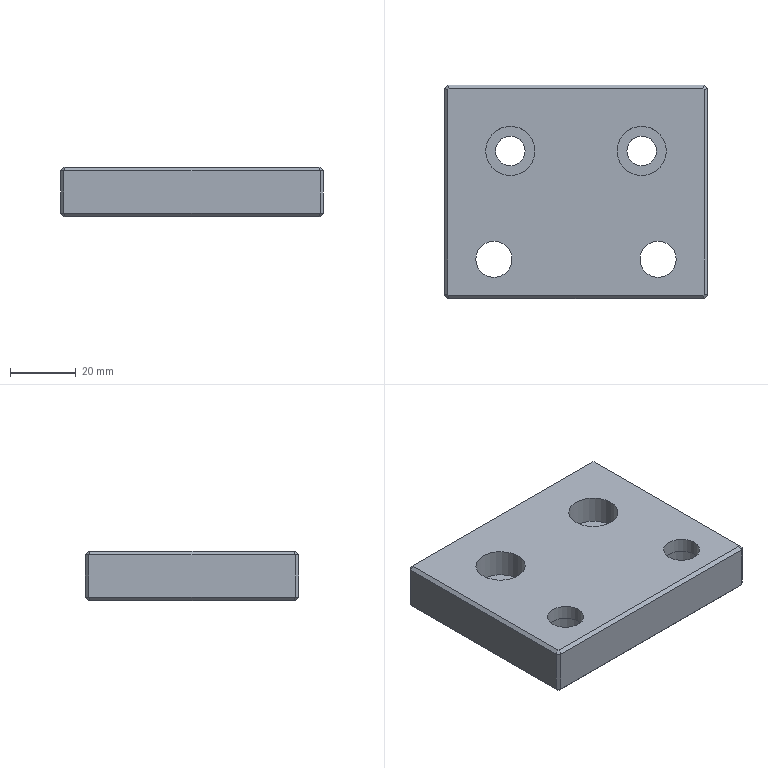Part | NX | 1 solid | 38 faces | box 80 x 65 x 15 mm | volume 67600 mm3 | plane 30 | cylinder 8 | commonest cylinder face diameters 9 x2 11 x2 15 x2 18 x2
STEP:
#1=CARTESIAN_POINT('',(40.,19.,1.));
#2=VERTEX_POINT('',#1);
#3=CARTESIAN_POINT('',(40.,19.,14.));
#4=VERTEX_POINT('',#3);
#5=CARTESIAN_POINT('',(40.,19.,15.));
#6=DIRECTION('',(0.,0.,1.));
#7=VECTOR('',#6,1000.);
#8=LINE('',#5,#7);
#9=EDGE_CURVE('',#2,#4,#8,.T.);
#10=ORIENTED_EDGE('',*,*,#9,.T.);
#11=CARTESIAN_POINT('',(40.,-44.,14.));
#12=VERTEX_POINT('',#11);
#13=CARTESIAN_POINT('',(40.,20.,14.));
#14=DIRECTION('',(0.,-1.,0.));
#15=VECTOR('',#14,1000.);
#16=LINE('',#13,#15);
#17=EDGE_CURVE('',#4,#12,#16,.T.);
#18=ORIENTED_EDGE('',*,*,#17,.T.);
#19=CARTESIAN_POINT('',(40.,-44.,1.));
#20=VERTEX_POINT('',#19);
#21=CARTESIAN_POINT('',(40.,-44.,15.));
#22=DIRECTION('',(0.,0.,-1.));
#23=VECTOR('',#22,1000.);
#24=LINE('',#21,#23);
#25=EDGE_CURVE('',#12,#20,#24,.T.);
#26=ORIENTED_EDGE('',*,*,#25,.T.);
#27=CARTESIAN_POINT('',(40.,19.,1.));
#28=DIRECTION('',(0.,1.,0.));
#29=VECTOR('',#28,1000.);
#30=LINE('',#27,#29);
#31=EDGE_CURVE('',#20,#2,#30,.T.);
#32=ORIENTED_EDGE('',*,*,#31,.T.);
#33=EDGE_LOOP('',(#10,#18,#26,#32));
#34=FACE_BOUND('',#33,.T.);
#35=CARTESIAN_POINT('',(40.,20.,15.));
#36=DIRECTION('',(-1.,0.,0.));
#37=DIRECTION('',(0.,-1.,0.));
#38=AXIS2_PLACEMENT_3D('',#35,#36,#37);
#39=PLANE('',#38);
#40=ADVANCED_FACE('',(#34),#39,.F.);
#41=CARTESIAN_POINT('',(-39.,20.,1.));
#42=VERTEX_POINT('',#41);
#43=CARTESIAN_POINT('',(-39.,20.,14.));
#44=VERTEX_POINT('',#43);
#45=CARTESIAN_POINT('',(-39.,20.,15.));
#46=DIRECTION('',(0.,0.,1.));
#47=VECTOR('',#46,1000.);
#48=LINE('',#45,#47);
#49=EDGE_CURVE('',#42,#44,#48,.T.);
#50=ORIENTED_EDGE('',*,*,#49,.T.);
#51=CARTESIAN_POINT('',(39.,20.,14.));
#52=VERTEX_POINT('',#51);
#53=CARTESIAN_POINT('',(40.,20.,14.));
#54=DIRECTION('',(1.,0.,0.));
#55=VECTOR('',#54,1000.);
#56=LINE('',#53,#55);
#57=EDGE_CURVE('',#44,#52,#56,.T.);
#58=ORIENTED_EDGE('',*,*,#57,.T.);
#59=CARTESIAN_POINT('',(39.,20.,1.));
#60=VERTEX_POINT('',#59);
#61=CARTESIAN_POINT('',(39.,20.,15.));
#62=DIRECTION('',(0.,0.,-1.));
#63=VECTOR('',#62,1000.);
#64=LINE('',#61,#63);
#65=EDGE_CURVE('',#52,#60,#64,.T.);
#66=ORIENTED_EDGE('',*,*,#65,.T.);
#67=CARTESIAN_POINT('',(-39.,20.,1.));
#68=DIRECTION('',(-1.,0.,0.));
#69=VECTOR('',#68,1000.);
#70=LINE('',#67,#69);
#71=EDGE_CURVE('',#60,#42,#70,.T.);
#72=ORIENTED_EDGE('',*,*,#71,.T.);
#73=EDGE_LOOP('',(#50,#58,#66,#72));
#74=FACE_BOUND('',#73,.T.);
#75=CARTESIAN_POINT('',(40.,20.,15.));
#76=DIRECTION('',(0.,-1.,0.));
#77=DIRECTION('',(0.,0.,-1.));
#78=AXIS2_PLACEMENT_3D('',#75,#76,#77);
#79=PLANE('',#78);
#80=ADVANCED_FACE('',(#74),#79,.F.);
#81=CARTESIAN_POINT('',(-40.,-44.,1.));
#82=VERTEX_POINT('',#81);
#83=CARTESIAN_POINT('',(-40.,-44.,14.));
#84=VERTEX_POINT('',#83);
#85=CARTESIAN_POINT('',(-40.,-44.,15.));
#86=DIRECTION('',(0.,0.,1.));
#87=VECTOR('',#86,1000.);
#88=LINE('',#85,#87);
#89=EDGE_CURVE('',#82,#84,#88,.T.);
#90=ORIENTED_EDGE('',*,*,#89,.T.);
#91=CARTESIAN_POINT('',(-40.,19.,14.));
#92=VERTEX_POINT('',#91);
#93=CARTESIAN_POINT('',(-40.,20.,14.));
#94=DIRECTION('',(0.,1.,0.));
#95=VECTOR('',#94,1000.);
#96=LINE('',#93,#95);
#97=EDGE_CURVE('',#84,#92,#96,.T.);
#98=ORIENTED_EDGE('',*,*,#97,.T.);
#99=CARTESIAN_POINT('',(-40.,19.,1.));
#100=VERTEX_POINT('',#99);
#101=CARTESIAN_POINT('',(-40.,19.,15.));
#102=DIRECTION('',(0.,0.,-1.));
#103=VECTOR('',#102,1000.);
#104=LINE('',#101,#103);
#105=EDGE_CURVE('',#92,#100,#104,.T.);
#106=ORIENTED_EDGE('',*,*,#105,.T.);
#107=CARTESIAN_POINT('',(-40.,-44.,1.));
#108=DIRECTION('',(0.,-1.,0.));
#109=VECTOR('',#108,1000.);
#110=LINE('',#107,#109);
#111=EDGE_CURVE('',#100,#82,#110,.T.);
#112=ORIENTED_EDGE('',*,*,#111,.T.);
#113=EDGE_LOOP('',(#90,#98,#106,#112));
#114=FACE_BOUND('',#113,.T.);
#115=CARTESIAN_POINT('',(-40.,20.,15.));
#116=DIRECTION('',(1.,0.,0.));
#117=DIRECTION('',(0.,1.,0.));
#118=AXIS2_PLACEMENT_3D('',#115,#116,#117);
#119=PLANE('',#118);
#120=ADVANCED_FACE('',(#114),#119,.F.);
#121=CARTESIAN_POINT('',(39.,-45.,1.));
#122=VERTEX_POINT('',#121);
#123=CARTESIAN_POINT('',(39.,-45.,14.));
#124=VERTEX_POINT('',#123);
#125=CARTESIAN_POINT('',(39.,-45.,15.));
#126=DIRECTION('',(0.,0.,1.));
#127=VECTOR('',#126,1000.);
#128=LINE('',#125,#127);
#129=EDGE_CURVE('',#122,#124,#128,.T.);
#130=ORIENTED_EDGE('',*,*,#129,.T.);
#131=CARTESIAN_POINT('',(-39.,-45.,14.));
#132=VERTEX_POINT('',#131);
#133=CARTESIAN_POINT('',(40.,-45.,14.));
#134=DIRECTION('',(-1.,0.,0.));
#135=VECTOR('',#134,1000.);
#136=LINE('',#133,#135);
#137=EDGE_CURVE('',#124,#132,#136,.T.);
#138=ORIENTED_EDGE('',*,*,#137,.T.);
#139=CARTESIAN_POINT('',(-39.,-45.,1.));
#140=VERTEX_POINT('',#139);
#141=CARTESIAN_POINT('',(-39.,-45.,15.));
#142=DIRECTION('',(0.,0.,-1.));
#143=VECTOR('',#142,1000.);
#144=LINE('',#141,#143);
#145=EDGE_CURVE('',#132,#140,#144,.T.);
#146=ORIENTED_EDGE('',*,*,#145,.T.);
#147=CARTESIAN_POINT('',(39.,-45.,1.));
#148=DIRECTION('',(1.,0.,0.));
#149=VECTOR('',#148,1000.);
#150=LINE('',#147,#149);
#151=EDGE_CURVE('',#140,#122,#150,.T.);
#152=ORIENTED_EDGE('',*,*,#151,.T.);
#153=EDGE_LOOP('',(#130,#138,#146,#152));
#154=FACE_BOUND('',#153,.T.);
#155=CARTESIAN_POINT('',(40.,-45.,15.));
#156=DIRECTION('',(0.,1.,0.));
#157=DIRECTION('',(0.,0.,1.));
#158=AXIS2_PLACEMENT_3D('',#155,#156,#157);
#159=PLANE('',#158);
#160=ADVANCED_FACE('',(#154),#159,.F.);
#161=CARTESIAN_POINT('',(-38.586,-44.,15.));
#162=VERTEX_POINT('',#161);
#163=CARTESIAN_POINT('',(38.586,-44.,15.));
#164=VERTEX_POINT('',#163);
#165=CARTESIAN_POINT('',(0.,-44.,15.));
#166=DIRECTION('',(1.,0.,0.));
#167=VECTOR('',#166,1000.);
#168=LINE('',#165,#167);
#169=EDGE_CURVE('',#162,#164,#168,.T.);
#170=ORIENTED_EDGE('',*,*,#169,.T.);
#171=CARTESIAN_POINT('',(39.,-43.586,15.));
#172=VERTEX_POINT('',#171);
#173=CARTESIAN_POINT('',(39.293,-43.293,15.));
#174=DIRECTION('',(0.7071,0.7071,0.));
#175=VECTOR('',#174,1000.);
#176=LINE('',#173,#175);
#177=EDGE_CURVE('',#164,#172,#176,.T.);
#178=ORIENTED_EDGE('',*,*,#177,.T.);
#179=CARTESIAN_POINT('',(39.,18.586,15.));
#180=VERTEX_POINT('',#179);
#181=CARTESIAN_POINT('',(39.,0.,15.));
#182=DIRECTION('',(0.,1.,0.));
#183=VECTOR('',#182,1000.);
#184=LINE('',#181,#183);
#185=EDGE_CURVE('',#172,#180,#184,.T.);
#186=ORIENTED_EDGE('',*,*,#185,.T.);
#187=CARTESIAN_POINT('',(38.586,19.,15.));
#188=VERTEX_POINT('',#187);
#189=CARTESIAN_POINT('',(38.293,19.293,15.));
#190=DIRECTION('',(-0.7071,0.7071,0.));
#191=VECTOR('',#190,1000.);
#192=LINE('',#189,#191);
#193=EDGE_CURVE('',#180,#188,#192,.T.);
#194=ORIENTED_EDGE('',*,*,#193,.T.);
#195=CARTESIAN_POINT('',(-38.586,19.,15.));
#196=VERTEX_POINT('',#195);
#197=CARTESIAN_POINT('',(0.,19.,15.));
#198=DIRECTION('',(-1.,0.,0.));
#199=VECTOR('',#198,1000.);
#200=LINE('',#197,#199);
#201=EDGE_CURVE('',#188,#196,#200,.T.);
#202=ORIENTED_EDGE('',*,*,#201,.T.);
#203=CARTESIAN_POINT('',(-39.,18.586,15.));
#204=VERTEX_POINT('',#203);
#205=CARTESIAN_POINT('',(-39.293,18.293,15.));
#206=DIRECTION('',(-0.7071,-0.7071,0.));
#207=VECTOR('',#206,1000.);
#208=LINE('',#205,#207);
#209=EDGE_CURVE('',#196,#204,#208,.T.);
#210=ORIENTED_EDGE('',*,*,#209,.T.);
#211=CARTESIAN_POINT('',(-39.,-43.586,15.));
#212=VERTEX_POINT('',#211);
#213=CARTESIAN_POINT('',(-39.,0.,15.));
#214=DIRECTION('',(0.,-1.,0.));
#215=VECTOR('',#214,1000.);
#216=LINE('',#213,#215);
#217=EDGE_CURVE('',#204,#212,#216,.T.);
#218=ORIENTED_EDGE('',*,*,#217,.T.);
#219=CARTESIAN_POINT('',(-38.293,-44.293,15.));
#220=DIRECTION('',(0.7071,-0.7071,0.));
#221=VECTOR('',#220,1000.);
#222=LINE('',#219,#221);
#223=EDGE_CURVE('',#212,#162,#222,.T.);
#224=ORIENTED_EDGE('',*,*,#223,.T.);
#225=EDGE_LOOP('',(#170,#178,#186,#194,#202,#210,#218,#224));
#226=FACE_BOUND('',#225,.T.);
#227=CARTESIAN_POINT('',(19.5,-33.,15.));
#228=VERTEX_POINT('',#227);
#229=CARTESIAN_POINT('',(25.,-33.,15.));
#230=DIRECTION('',(0.,0.,-1.));
#231=DIRECTION('',(-1.,0.,0.));
#232=AXIS2_PLACEMENT_3D('',#229,#230,#231);
#233=CIRCLE('',#232,5.5);
#234=EDGE_CURVE('',#228,#228,#233,.T.);
#235=ORIENTED_EDGE('',*,*,#234,.T.);
#236=EDGE_LOOP('',(#235));
#237=FACE_BOUND('',#236,.T.);
#238=CARTESIAN_POINT('',(-30.5,-33.,15.));
#239=VERTEX_POINT('',#238);
#240=CARTESIAN_POINT('',(-25.,-33.,15.));
#241=DIRECTION('',(0.,0.,-1.));
#242=DIRECTION('',(-1.,0.,0.));
#243=AXIS2_PLACEMENT_3D('',#240,#241,#242);
#244=CIRCLE('',#243,5.5);
#245=EDGE_CURVE('',#239,#239,#244,.T.);
#246=ORIENTED_EDGE('',*,*,#245,.T.);
#247=EDGE_LOOP('',(#246));
#248=FACE_BOUND('',#247,.T.);
#249=CARTESIAN_POINT('',(-12.5,0.,15.));
#250=VERTEX_POINT('',#249);
#251=CARTESIAN_POINT('',(-20.,0.,15.));
#252=DIRECTION('',(0.,0.,1.));
#253=DIRECTION('',(1.,0.,0.));
#254=AXIS2_PLACEMENT_3D('',#251,#252,#253);
#255=CIRCLE('',#254,7.5);
#256=EDGE_CURVE('',#250,#250,#255,.T.);
#257=ORIENTED_EDGE('',*,*,#256,.F.);
#258=EDGE_LOOP('',(#257));
#259=FACE_BOUND('',#258,.T.);
#260=CARTESIAN_POINT('',(27.5,0.,15.));
#261=VERTEX_POINT('',#260);
#262=CARTESIAN_POINT('',(20.,0.,15.));
#263=DIRECTION('',(0.,0.,1.));
#264=DIRECTION('',(1.,0.,0.));
#265=AXIS2_PLACEMENT_3D('',#262,#263,#264);
#266=CIRCLE('',#265,7.5);
#267=EDGE_CURVE('',#261,#261,#266,.T.);
#268=ORIENTED_EDGE('',*,*,#267,.F.);
#269=EDGE_LOOP('',(#268));
#270=FACE_BOUND('',#269,.T.);
#271=CARTESIAN_POINT('',(0.,0.,15.));
#272=DIRECTION('',(0.,0.,-1.));
#273=DIRECTION('',(-1.,0.,0.));
#274=AXIS2_PLACEMENT_3D('',#271,#272,#273);
#275=PLANE('',#274);
#276=ADVANCED_FACE('',(#226,#237,#248,#259,#270),#275,.F.);
#277=CARTESIAN_POINT('',(-38.586,19.,0.));
#278=VERTEX_POINT('',#277);
#279=CARTESIAN_POINT('',(38.586,19.,0.));
#280=VERTEX_POINT('',#279);
#281=CARTESIAN_POINT('',(39.,19.,0.));
#282=DIRECTION('',(1.,0.,0.));
#283=VECTOR('',#282,1000.);
#284=LINE('',#281,#283);
#285=EDGE_CURVE('',#278,#280,#284,.T.);
#286=ORIENTED_EDGE('',*,*,#285,.T.);
#287=CARTESIAN_POINT('',(39.,18.586,0.));
#288=VERTEX_POINT('',#287);
#289=CARTESIAN_POINT('',(28.793,28.793,0.));
#290=DIRECTION('',(0.7071,-0.7071,0.));
#291=VECTOR('',#290,1000.);
#292=LINE('',#289,#291);
#293=EDGE_CURVE('',#280,#288,#292,.T.);
#294=ORIENTED_EDGE('',*,*,#293,.T.);
#295=CARTESIAN_POINT('',(39.,-43.586,0.));
#296=VERTEX_POINT('',#295);
#297=CARTESIAN_POINT('',(39.,-44.,0.));
#298=DIRECTION('',(0.,-1.,0.));
#299=VECTOR('',#298,1000.);
#300=LINE('',#297,#299);
#301=EDGE_CURVE('',#288,#296,#300,.T.);
#302=ORIENTED_EDGE('',*,*,#301,.T.);
#303=CARTESIAN_POINT('',(38.586,-44.,0.));
#304=VERTEX_POINT('',#303);
#305=CARTESIAN_POINT('',(41.293,-41.293,0.));
#306=DIRECTION('',(-0.7071,-0.7071,0.));
#307=VECTOR('',#306,1000.);
#308=LINE('',#305,#307);
#309=EDGE_CURVE('',#296,#304,#308,.T.);
#310=ORIENTED_EDGE('',*,*,#309,.T.);
#311=CARTESIAN_POINT('',(-38.586,-44.,0.));
#312=VERTEX_POINT('',#311);
#313=CARTESIAN_POINT('',(-39.,-44.,0.));
#314=DIRECTION('',(-1.,0.,0.));
#315=VECTOR('',#314,1000.);
#316=LINE('',#313,#315);
#317=EDGE_CURVE('',#304,#312,#316,.T.);
#318=ORIENTED_EDGE('',*,*,#317,.T.);
#319=CARTESIAN_POINT('',(-39.,-43.586,0.));
#320=VERTEX_POINT('',#319);
#321=CARTESIAN_POINT('',(-41.293,-41.293,0.));
#322=DIRECTION('',(-0.7071,0.7071,0.));
#323=VECTOR('',#322,1000.);
#324=LINE('',#321,#323);
#325=EDGE_CURVE('',#312,#320,#324,.T.);
#326=ORIENTED_EDGE('',*,*,#325,.T.);
#327=CARTESIAN_POINT('',(-39.,18.586,0.));
#328=VERTEX_POINT('',#327);
#329=CARTESIAN_POINT('',(-39.,19.,0.));
#330=DIRECTION('',(0.,1.,0.));
#331=VECTOR('',#330,1000.);
#332=LINE('',#329,#331);
#333=EDGE_CURVE('',#320,#328,#332,.T.);
#334=ORIENTED_EDGE('',*,*,#333,.T.);
#335=CARTESIAN_POINT('',(-28.793,28.793,0.));
#336=DIRECTION('',(0.7071,0.7071,0.));
#337=VECTOR('',#336,1000.);
#338=LINE('',#335,#337);
#339=EDGE_CURVE('',#328,#278,#338,.T.);
#340=ORIENTED_EDGE('',*,*,#339,.T.);
#341=EDGE_LOOP('',(#286,#294,#302,#310,#318,#326,#334,#340));
#342=FACE_BOUND('',#341,.T.);
#343=CARTESIAN_POINT('',(16.,-33.,0.));
#344=VERTEX_POINT('',#343);
#345=CARTESIAN_POINT('',(25.,-33.,0.));
#346=DIRECTION('',(0.,0.,-1.));
#347=DIRECTION('',(-1.,0.,0.));
#348=AXIS2_PLACEMENT_3D('',#345,#346,#347);
#349=CIRCLE('',#348,9.);
#350=EDGE_CURVE('',#344,#344,#349,.T.);
#351=ORIENTED_EDGE('',*,*,#350,.F.);
#352=EDGE_LOOP('',(#351));
#353=FACE_BOUND('',#352,.T.);
#354=CARTESIAN_POINT('',(-34.,-33.,0.));
#355=VERTEX_POINT('',#354);
#356=CARTESIAN_POINT('',(-25.,-33.,0.));
#357=DIRECTION('',(0.,0.,-1.));
#358=DIRECTION('',(-1.,0.,0.));
#359=AXIS2_PLACEMENT_3D('',#356,#357,#358);
#360=CIRCLE('',#359,9.);
#361=EDGE_CURVE('',#355,#355,#360,.T.);
#362=ORIENTED_EDGE('',*,*,#361,.F.);
#363=EDGE_LOOP('',(#362));
#364=FACE_BOUND('',#363,.T.);
#365=CARTESIAN_POINT('',(-15.5,0.,0.));
#366=VERTEX_POINT('',#365);
#367=CARTESIAN_POINT('',(-20.,0.,0.));
#368=DIRECTION('',(0.,0.,1.));
#369=DIRECTION('',(1.,0.,0.));
#370=AXIS2_PLACEMENT_3D('',#367,#368,#369);
#371=CIRCLE('',#370,4.5);
#372=EDGE_CURVE('',#366,#366,#371,.T.);
#373=ORIENTED_EDGE('',*,*,#372,.T.);
#374=EDGE_LOOP('',(#373));
#375=FACE_BOUND('',#374,.T.);
#376=CARTESIAN_POINT('',(24.5,0.,0.));
#377=VERTEX_POINT('',#376);
#378=CARTESIAN_POINT('',(20.,0.,0.));
#379=DIRECTION('',(0.,0.,1.));
#380=DIRECTION('',(1.,0.,0.));
#381=AXIS2_PLACEMENT_3D('',#378,#379,#380);
#382=CIRCLE('',#381,4.5);
#383=EDGE_CURVE('',#377,#377,#382,.T.);
#384=ORIENTED_EDGE('',*,*,#383,.T.);
#385=EDGE_LOOP('',(#384));
#386=FACE_BOUND('',#385,.T.);
#387=CARTESIAN_POINT('',(0.,0.,0.));
#388=DIRECTION('',(0.,0.,-1.));
#389=DIRECTION('',(-1.,0.,0.));
#390=AXIS2_PLACEMENT_3D('',#387,#388,#389);
#391=PLANE('',#390);
#392=ADVANCED_FACE('',(#342,#353,#364,#375,#386),#391,.T.);
#393=ORIENTED_EDGE('',*,*,#383,.F.);
#394=EDGE_LOOP('',(#393));
#395=FACE_BOUND('',#394,.T.);
#396=CARTESIAN_POINT('',(24.5,0.,6.4));
#397=VERTEX_POINT('',#396);
#398=CARTESIAN_POINT('',(20.,0.,6.4));
#399=DIRECTION('',(0.,0.,1.));
#400=DIRECTION('',(1.,0.,0.));
#401=AXIS2_PLACEMENT_3D('',#398,#399,#400);
#402=CIRCLE('',#401,4.5);
#403=EDGE_CURVE('',#397,#397,#402,.T.);
#404=ORIENTED_EDGE('',*,*,#403,.T.);
#405=EDGE_LOOP('',(#404));
#406=FACE_BOUND('',#405,.T.);
#407=CARTESIAN_POINT('',(20.,0.,15.));
#408=DIRECTION('',(0.,0.,1.));
#409=DIRECTION('',(1.,0.,0.));
#410=AXIS2_PLACEMENT_3D('',#407,#408,#409);
#411=CYLINDRICAL_SURFACE('',#410,4.5);
#412=ADVANCED_FACE('',(#395,#406),#411,.F.);
#413=ORIENTED_EDGE('',*,*,#403,.F.);
#414=EDGE_LOOP('',(#413));
#415=FACE_BOUND('',#414,.T.);
#416=CARTESIAN_POINT('',(27.5,0.,6.4));
#417=VERTEX_POINT('',#416);
#418=CARTESIAN_POINT('',(20.,0.,6.4));
#419=DIRECTION('',(0.,0.,1.));
#420=DIRECTION('',(1.,0.,0.));
#421=AXIS2_PLACEMENT_3D('',#418,#419,#420);
#422=CIRCLE('',#421,7.5);
#423=EDGE_CURVE('',#417,#417,#422,.T.);
#424=ORIENTED_EDGE('',*,*,#423,.T.);
#425=EDGE_LOOP('',(#424));
#426=FACE_BOUND('',#425,.T.);
#427=CARTESIAN_POINT('',(24.5,0.,6.4));
#428=DIRECTION('',(0.,0.,-1.));
#429=DIRECTION('',(-1.,0.,0.));
#430=AXIS2_PLACEMENT_3D('',#427,#428,#429);
#431=PLANE('',#430);
#432=ADVANCED_FACE('',(#415,#426),#431,.F.);
#433=ORIENTED_EDGE('',*,*,#423,.F.);
#434=EDGE_LOOP('',(#433));
#435=FACE_BOUND('',#434,.T.);
#436=ORIENTED_EDGE('',*,*,#267,.T.);
#437=EDGE_LOOP('',(#436));
#438=FACE_BOUND('',#437,.T.);
#439=CARTESIAN_POINT('',(20.,0.,15.));
#440=DIRECTION('',(0.,0.,1.));
#441=DIRECTION('',(1.,0.,0.));
#442=AXIS2_PLACEMENT_3D('',#439,#440,#441);
#443=CYLINDRICAL_SURFACE('',#442,7.5);
#444=ADVANCED_FACE('',(#435,#438),#443,.F.);
#445=ORIENTED_EDGE('',*,*,#372,.F.);
#446=EDGE_LOOP('',(#445));
#447=FACE_BOUND('',#446,.T.);
#448=CARTESIAN_POINT('',(-15.5,0.,6.4));
#449=VERTEX_POINT('',#448);
#450=CARTESIAN_POINT('',(-20.,0.,6.4));
#451=DIRECTION('',(0.,0.,1.));
#452=DIRECTION('',(1.,0.,0.));
#453=AXIS2_PLACEMENT_3D('',#450,#451,#452);
#454=CIRCLE('',#453,4.5);
#455=EDGE_CURVE('',#449,#449,#454,.T.);
#456=ORIENTED_EDGE('',*,*,#455,.T.);
#457=EDGE_LOOP('',(#456));
#458=FACE_BOUND('',#457,.T.);
#459=CARTESIAN_POINT('',(-20.,0.,15.));
#460=DIRECTION('',(0.,0.,1.));
#461=DIRECTION('',(1.,0.,0.));
#462=AXIS2_PLACEMENT_3D('',#459,#460,#461);
#463=CYLINDRICAL_SURFACE('',#462,4.5);
#464=ADVANCED_FACE('',(#447,#458),#463,.F.);
#465=ORIENTED_EDGE('',*,*,#455,.F.);
#466=EDGE_LOOP('',(#465));
#467=FACE_BOUND('',#466,.T.);
#468=CARTESIAN_POINT('',(-12.5,0.,6.4));
#469=VERTEX_POINT('',#468);
#470=CARTESIAN_POINT('',(-20.,0.,6.4));
#471=DIRECTION('',(0.,0.,1.));
#472=DIRECTION('',(1.,0.,0.));
#473=AXIS2_PLACEMENT_3D('',#470,#471,#472);
#474=CIRCLE('',#473,7.5);
#475=EDGE_CURVE('',#469,#469,#474,.T.);
#476=ORIENTED_EDGE('',*,*,#475,.T.);
#477=EDGE_LOOP('',(#476));
#478=FACE_BOUND('',#477,.T.);
#479=CARTESIAN_POINT('',(-15.5,0.,6.4));
#480=DIRECTION('',(0.,0.,-1.));
#481=DIRECTION('',(-1.,0.,0.));
#482=AXIS2_PLACEMENT_3D('',#479,#480,#481);
#483=PLANE('',#482);
#484=ADVANCED_FACE('',(#467,#478),#483,.F.);
#485=ORIENTED_EDGE('',*,*,#475,.F.);
#486=EDGE_LOOP('',(#485));
#487=FACE_BOUND('',#486,.T.);
#488=ORIENTED_EDGE('',*,*,#256,.T.);
#489=EDGE_LOOP('',(#488));
#490=FACE_BOUND('',#489,.T.);
#491=CARTESIAN_POINT('',(-20.,0.,15.));
#492=DIRECTION('',(0.,0.,1.));
#493=DIRECTION('',(1.,0.,0.));
#494=AXIS2_PLACEMENT_3D('',#491,#492,#493);
#495=CYLINDRICAL_SURFACE('',#494,7.5);
#496=ADVANCED_FACE('',(#487,#490),#495,.F.);
#497=ORIENTED_EDGE('',*,*,#245,.F.);
#498=EDGE_LOOP('',(#497));
#499=FACE_BOUND('',#498,.T.);
#500=CARTESIAN_POINT('',(-30.5,-33.,10.6));
#501=VERTEX_POINT('',#500);
#502=CARTESIAN_POINT('',(-25.,-33.,10.6));
#503=DIRECTION('',(0.,0.,-1.));
#504=DIRECTION('',(-1.,0.,0.));
#505=AXIS2_PLACEMENT_3D('',#502,#503,#504);
#506=CIRCLE('',#505,5.5);
#507=EDGE_CURVE('',#501,#501,#506,.T.);
#508=ORIENTED_EDGE('',*,*,#507,.T.);
#509=EDGE_LOOP('',(#508));
#510=FACE_BOUND('',#509,.T.);
#511=CARTESIAN_POINT('',(-25.,-33.,0.));
#512=DIRECTION('',(0.,0.,-1.));
#513=DIRECTION('',(-1.,0.,0.));
#514=AXIS2_PLACEMENT_3D('',#511,#512,#513);
#515=CYLINDRICAL_SURFACE('',#514,5.5);
#516=ADVANCED_FACE('',(#499,#510),#515,.F.);
#517=ORIENTED_EDGE('',*,*,#507,.F.);
#518=EDGE_LOOP('',(#517));
#519=FACE_BOUND('',#518,.T.);
#520=CARTESIAN_POINT('',(-34.,-33.,10.6));
#521=VERTEX_POINT('',#520);
#522=CARTESIAN_POINT('',(-25.,-33.,10.6));
#523=DIRECTION('',(0.,0.,-1.));
#524=DIRECTION('',(-1.,0.,0.));
#525=AXIS2_PLACEMENT_3D('',#522,#523,#524);
#526=CIRCLE('',#525,9.);
#527=EDGE_CURVE('',#521,#521,#526,.T.);
#528=ORIENTED_EDGE('',*,*,#527,.T.);
#529=EDGE_LOOP('',(#528));
#530=FACE_BOUND('',#529,.T.);
#531=CARTESIAN_POINT('',(-19.5,-33.,10.6));
#532=DIRECTION('',(0.,0.,1.));
#533=DIRECTION('',(1.,0.,0.));
#534=AXIS2_PLACEMENT_3D('',#531,#532,#533);
#535=PLANE('',#534);
#536=ADVANCED_FACE('',(#519,#530),#535,.F.);
#537=ORIENTED_EDGE('',*,*,#527,.F.);
#538=EDGE_LOOP('',(#537));
#539=FACE_BOUND('',#538,.T.);
#540=ORIENTED_EDGE('',*,*,#361,.T.);
#541=EDGE_LOOP('',(#540));
#542=FACE_BOUND('',#541,.T.);
#543=CARTESIAN_POINT('',(-25.,-33.,0.));
#544=DIRECTION('',(0.,0.,-1.));
#545=DIRECTION('',(-1.,0.,0.));
#546=AXIS2_PLACEMENT_3D('',#543,#544,#545);
#547=CYLINDRICAL_SURFACE('',#546,9.);
#548=ADVANCED_FACE('',(#539,#542),#547,.F.);
#549=ORIENTED_EDGE('',*,*,#234,.F.);
#550=EDGE_LOOP('',(#549));
#551=FACE_BOUND('',#550,.T.);
#552=CARTESIAN_POINT('',(19.5,-33.,10.6));
#553=VERTEX_POINT('',#552);
#554=CARTESIAN_POINT('',(25.,-33.,10.6));
#555=DIRECTION('',(0.,0.,-1.));
#556=DIRECTION('',(-1.,0.,0.));
#557=AXIS2_PLACEMENT_3D('',#554,#555,#556);
#558=CIRCLE('',#557,5.5);
#559=EDGE_CURVE('',#553,#553,#558,.T.);
#560=ORIENTED_EDGE('',*,*,#559,.T.);
#561=EDGE_LOOP('',(#560));
#562=FACE_BOUND('',#561,.T.);
#563=CARTESIAN_POINT('',(25.,-33.,0.));
#564=DIRECTION('',(0.,0.,-1.));
#565=DIRECTION('',(-1.,0.,0.));
#566=AXIS2_PLACEMENT_3D('',#563,#564,#565);
#567=CYLINDRICAL_SURFACE('',#566,5.5);
#568=ADVANCED_FACE('',(#551,#562),#567,.F.);
#569=ORIENTED_EDGE('',*,*,#559,.F.);
#570=EDGE_LOOP('',(#569));
#571=FACE_BOUND('',#570,.T.);
#572=CARTESIAN_POINT('',(16.,-33.,10.6));
#573=VERTEX_POINT('',#572);
#574=CARTESIAN_POINT('',(25.,-33.,10.6));
#575=DIRECTION('',(0.,0.,-1.));
#576=DIRECTION('',(-1.,0.,0.));
#577=AXIS2_PLACEMENT_3D('',#574,#575,#576);
#578=CIRCLE('',#577,9.);
#579=EDGE_CURVE('',#573,#573,#578,.T.);
#580=ORIENTED_EDGE('',*,*,#579,.T.);
#581=EDGE_LOOP('',(#580));
#582=FACE_BOUND('',#581,.T.);
#583=CARTESIAN_POINT('',(30.5,-33.,10.6));
#584=DIRECTION('',(0.,0.,1.));
#585=DIRECTION('',(1.,0.,0.));
#586=AXIS2_PLACEMENT_3D('',#583,#584,#585);
#587=PLANE('',#586);
#588=ADVANCED_FACE('',(#571,#582),#587,.F.);
#589=ORIENTED_EDGE('',*,*,#579,.F.);
#590=EDGE_LOOP('',(#589));
#591=FACE_BOUND('',#590,.T.);
#592=ORIENTED_EDGE('',*,*,#350,.T.);
#593=EDGE_LOOP('',(#592));
#594=FACE_BOUND('',#593,.T.);
#595=CARTESIAN_POINT('',(25.,-33.,0.));
#596=DIRECTION('',(0.,0.,-1.));
#597=DIRECTION('',(-1.,0.,0.));
#598=AXIS2_PLACEMENT_3D('',#595,#596,#597);
#599=CYLINDRICAL_SURFACE('',#598,9.);
#600=ADVANCED_FACE('',(#591,#594),#599,.F.);
#601=ORIENTED_EDGE('',*,*,#25,.F.);
#602=CARTESIAN_POINT('',(39.,-45.,14.));
#603=DIRECTION('',(0.7071,0.7071,0.));
#604=VECTOR('',#603,1000.);
#605=LINE('',#602,#604);
#606=EDGE_CURVE('',#12,#124,#605,.F.);
#607=ORIENTED_EDGE('',*,*,#606,.T.);
#608=ORIENTED_EDGE('',*,*,#129,.F.);
#609=CARTESIAN_POINT('',(40.,-44.,1.));
#610=DIRECTION('',(-0.7071,-0.7071,0.));
#611=VECTOR('',#610,1000.);
#612=LINE('',#609,#611);
#613=EDGE_CURVE('',#122,#20,#612,.F.);
#614=ORIENTED_EDGE('',*,*,#613,.T.);
#615=EDGE_LOOP('',(#601,#607,#608,#614));
#616=FACE_BOUND('',#615,.T.);
#617=CARTESIAN_POINT('',(40.,-44.,15.));
#618=DIRECTION('',(-0.7071,0.7071,0.));
#619=DIRECTION('',(0.,0.,-1.));
#620=AXIS2_PLACEMENT_3D('',#617,#618,#619);
#621=PLANE('',#620);
#622=ADVANCED_FACE('',(#616),#621,.F.);
#623=ORIENTED_EDGE('',*,*,#65,.F.);
#624=CARTESIAN_POINT('',(40.,19.,14.));
#625=DIRECTION('',(-0.7071,0.7071,0.));
#626=VECTOR('',#625,1000.);
#627=LINE('',#624,#626);
#628=EDGE_CURVE('',#52,#4,#627,.F.);
#629=ORIENTED_EDGE('',*,*,#628,.T.);
#630=ORIENTED_EDGE('',*,*,#9,.F.);
#631=CARTESIAN_POINT('',(39.,20.,1.));
#632=DIRECTION('',(0.7071,-0.7071,0.));
#633=VECTOR('',#632,1000.);
#634=LINE('',#631,#633);
#635=EDGE_CURVE('',#2,#60,#634,.F.);
#636=ORIENTED_EDGE('',*,*,#635,.T.);
#637=EDGE_LOOP('',(#623,#629,#630,#636));
#638=FACE_BOUND('',#637,.T.);
#639=CARTESIAN_POINT('',(39.,20.,15.));
#640=DIRECTION('',(-0.7071,-0.7071,0.));
#641=DIRECTION('',(0.,0.,-1.));
#642=AXIS2_PLACEMENT_3D('',#639,#640,#641);
#643=PLANE('',#642);
#644=ADVANCED_FACE('',(#638),#643,.F.);
#645=ORIENTED_EDGE('',*,*,#105,.F.);
#646=CARTESIAN_POINT('',(-39.,20.,14.));
#647=DIRECTION('',(-0.7071,-0.7071,0.));
#648=VECTOR('',#647,1000.);
#649=LINE('',#646,#648);
#650=EDGE_CURVE('',#92,#44,#649,.F.);
#651=ORIENTED_EDGE('',*,*,#650,.T.);
#652=ORIENTED_EDGE('',*,*,#49,.F.);
#653=CARTESIAN_POINT('',(-40.,19.,1.));
#654=DIRECTION('',(0.7071,0.7071,0.));
#655=VECTOR('',#654,1000.);
#656=LINE('',#653,#655);
#657=EDGE_CURVE('',#42,#100,#656,.F.);
#658=ORIENTED_EDGE('',*,*,#657,.T.);
#659=EDGE_LOOP('',(#645,#651,#652,#658));
#660=FACE_BOUND('',#659,.T.);
#661=CARTESIAN_POINT('',(-40.,19.,15.));
#662=DIRECTION('',(0.7071,-0.7071,0.));
#663=DIRECTION('',(0.,0.,-1.));
#664=AXIS2_PLACEMENT_3D('',#661,#662,#663);
#665=PLANE('',#664);
#666=ADVANCED_FACE('',(#660),#665,.F.);
#667=ORIENTED_EDGE('',*,*,#145,.F.);
#668=CARTESIAN_POINT('',(-40.,-44.,14.));
#669=DIRECTION('',(0.7071,-0.7071,0.));
#670=VECTOR('',#669,1000.);
#671=LINE('',#668,#670);
#672=EDGE_CURVE('',#132,#84,#671,.F.);
#673=ORIENTED_EDGE('',*,*,#672,.T.);
#674=ORIENTED_EDGE('',*,*,#89,.F.);
#675=CARTESIAN_POINT('',(-39.,-45.,1.));
#676=DIRECTION('',(-0.7071,0.7071,0.));
#677=VECTOR('',#676,1000.);
#678=LINE('',#675,#677);
#679=EDGE_CURVE('',#82,#140,#678,.F.);
#680=ORIENTED_EDGE('',*,*,#679,.T.);
#681=EDGE_LOOP('',(#667,#673,#674,#680));
#682=FACE_BOUND('',#681,.T.);
#683=CARTESIAN_POINT('',(-39.,-45.,15.));
#684=DIRECTION('',(0.7071,0.7071,0.));
#685=DIRECTION('',(0.,0.,-1.));
#686=AXIS2_PLACEMENT_3D('',#683,#684,#685);
#687=PLANE('',#686);
#688=ADVANCED_FACE('',(#682),#687,.F.);
#689=CARTESIAN_POINT('',(-35.537,11.64,22.36));
#690=DIRECTION('',(0.2811,-0.6786,0.6786));
#691=VECTOR('',#690,1000.);
#692=LINE('',#689,#691);
#693=EDGE_CURVE('',#44,#196,#692,.T.);
#694=ORIENTED_EDGE('',*,*,#693,.F.);
#695=ORIENTED_EDGE('',*,*,#650,.F.);
#696=CARTESIAN_POINT('',(-36.247,17.445,17.753));
#697=DIRECTION('',(0.6786,-0.2811,0.6786));
#698=VECTOR('',#697,1000.);
#699=LINE('',#696,#698);
#700=EDGE_CURVE('',#204,#92,#699,.F.);
#701=ORIENTED_EDGE('',*,*,#700,.F.);
#702=ORIENTED_EDGE('',*,*,#209,.F.);
#703=EDGE_LOOP('',(#694,#695,#701,#702));
#704=FACE_BOUND('',#703,.T.);
#705=CARTESIAN_POINT('',(-28.793,28.793,15.));
#706=DIRECTION('',(0.5,-0.5,-0.7071));
#707=DIRECTION('',(-0.7071,-0.7071,0.));
#708=AXIS2_PLACEMENT_3D('',#705,#706,#707);
#709=PLANE('',#708);
#710=ADVANCED_FACE('',(#704),#709,.F.);
#711=ORIENTED_EDGE('',*,*,#700,.T.);
#712=ORIENTED_EDGE('',*,*,#97,.F.);
#713=CARTESIAN_POINT('',(-30.686,-40.142,23.314));
#714=DIRECTION('',(0.6786,0.2811,0.6786));
#715=VECTOR('',#714,1000.);
#716=LINE('',#713,#715);
#717=EDGE_CURVE('',#212,#84,#716,.F.);
#718=ORIENTED_EDGE('',*,*,#717,.F.);
#719=ORIENTED_EDGE('',*,*,#217,.F.);
#720=EDGE_LOOP('',(#711,#712,#718,#719));
#721=FACE_BOUND('',#720,.T.);
#722=CARTESIAN_POINT('',(-39.,0.,15.));
#723=DIRECTION('',(0.7071,0.,-0.7071));
#724=DIRECTION('',(0.,-1.,0.));
#725=AXIS2_PLACEMENT_3D('',#722,#723,#724);
#726=PLANE('',#725);
#727=ADVANCED_FACE('',(#721),#726,.F.);
#728=ORIENTED_EDGE('',*,*,#693,.T.);
#729=ORIENTED_EDGE('',*,*,#201,.F.);
#730=CARTESIAN_POINT('',(39.68,21.642,12.358));
#731=DIRECTION('',(-0.2811,-0.6786,0.6786));
#732=VECTOR('',#731,1000.);
#733=LINE('',#730,#732);
#734=EDGE_CURVE('',#52,#188,#733,.T.);
#735=ORIENTED_EDGE('',*,*,#734,.F.);
#736=ORIENTED_EDGE('',*,*,#57,.F.);
#737=EDGE_LOOP('',(#728,#729,#735,#736));
#738=FACE_BOUND('',#737,.T.);
#739=CARTESIAN_POINT('',(0.,19.,15.));
#740=DIRECTION('',(0.,-0.7071,-0.7071));
#741=DIRECTION('',(-1.,0.,0.));
#742=AXIS2_PLACEMENT_3D('',#739,#740,#741);
#743=PLANE('',#742);
#744=ADVANCED_FACE('',(#738),#743,.F.);
#745=ORIENTED_EDGE('',*,*,#717,.T.);
#746=ORIENTED_EDGE('',*,*,#672,.F.);
#747=CARTESIAN_POINT('',(-38.283,-43.27,15.73));
#748=DIRECTION('',(0.2811,0.6786,0.6786));
#749=VECTOR('',#748,1000.);
#750=LINE('',#747,#749);
#751=EDGE_CURVE('',#162,#132,#750,.F.);
#752=ORIENTED_EDGE('',*,*,#751,.F.);
#753=ORIENTED_EDGE('',*,*,#223,.F.);
#754=EDGE_LOOP('',(#745,#746,#752,#753));
#755=FACE_BOUND('',#754,.T.);
#756=CARTESIAN_POINT('',(-41.293,-41.293,15.));
#757=DIRECTION('',(0.5,0.5,-0.7071));
#758=DIRECTION('',(0.7071,-0.7071,0.));
#759=AXIS2_PLACEMENT_3D('',#756,#757,#758);
#760=PLANE('',#759);
#761=ADVANCED_FACE('',(#755),#760,.F.);
#762=ORIENTED_EDGE('',*,*,#734,.T.);
#763=ORIENTED_EDGE('',*,*,#193,.F.);
#764=CARTESIAN_POINT('',(36.247,17.445,17.753));
#765=DIRECTION('',(0.6786,0.2811,-0.6786));
#766=VECTOR('',#765,1000.);
#767=LINE('',#764,#766);
#768=EDGE_CURVE('',#4,#180,#767,.F.);
#769=ORIENTED_EDGE('',*,*,#768,.F.);
#770=ORIENTED_EDGE('',*,*,#628,.F.);
#771=EDGE_LOOP('',(#762,#763,#769,#770));
#772=FACE_BOUND('',#771,.T.);
#773=CARTESIAN_POINT('',(28.793,28.793,15.));
#774=DIRECTION('',(-0.5,-0.5,-0.7071));
#775=DIRECTION('',(-0.7071,0.7071,0.));
#776=AXIS2_PLACEMENT_3D('',#773,#774,#775);
#777=PLANE('',#776);
#778=ADVANCED_FACE('',(#772),#777,.F.);
#779=ORIENTED_EDGE('',*,*,#751,.T.);
#780=ORIENTED_EDGE('',*,*,#137,.F.);
#781=CARTESIAN_POINT('',(35.537,-36.64,22.36));
#782=DIRECTION('',(-0.2811,0.6786,0.6786));
#783=VECTOR('',#782,1000.);
#784=LINE('',#781,#783);
#785=EDGE_CURVE('',#164,#124,#784,.F.);
#786=ORIENTED_EDGE('',*,*,#785,.F.);
#787=ORIENTED_EDGE('',*,*,#169,.F.);
#788=EDGE_LOOP('',(#779,#780,#786,#787));
#789=FACE_BOUND('',#788,.T.);
#790=CARTESIAN_POINT('',(0.,-44.,15.));
#791=DIRECTION('',(0.,0.7071,-0.7071));
#792=DIRECTION('',(1.,0.,0.));
#793=AXIS2_PLACEMENT_3D('',#790,#791,#792);
#794=PLANE('',#793);
#795=ADVANCED_FACE('',(#789),#794,.F.);
#796=ORIENTED_EDGE('',*,*,#768,.T.);
#797=ORIENTED_EDGE('',*,*,#185,.F.);
#798=CARTESIAN_POINT('',(30.686,-40.142,23.314));
#799=DIRECTION('',(0.6786,-0.2811,-0.6786));
#800=VECTOR('',#799,1000.);
#801=LINE('',#798,#800);
#802=EDGE_CURVE('',#12,#172,#801,.F.);
#803=ORIENTED_EDGE('',*,*,#802,.F.);
#804=ORIENTED_EDGE('',*,*,#17,.F.);
#805=EDGE_LOOP('',(#796,#797,#803,#804));
#806=FACE_BOUND('',#805,.T.);
#807=CARTESIAN_POINT('',(39.,0.,15.));
#808=DIRECTION('',(-0.7071,0.,-0.7071));
#809=DIRECTION('',(0.,1.,0.));
#810=AXIS2_PLACEMENT_3D('',#807,#808,#809);
#811=PLANE('',#810);
#812=ADVANCED_FACE('',(#806),#811,.F.);
#813=ORIENTED_EDGE('',*,*,#785,.T.);
#814=ORIENTED_EDGE('',*,*,#606,.F.);
#815=ORIENTED_EDGE('',*,*,#802,.T.);
#816=ORIENTED_EDGE('',*,*,#177,.F.);
#817=EDGE_LOOP('',(#813,#814,#815,#816));
#818=FACE_BOUND('',#817,.T.);
#819=CARTESIAN_POINT('',(41.293,-41.293,15.));
#820=DIRECTION('',(-0.5,0.5,-0.7071));
#821=DIRECTION('',(0.7071,0.7071,0.));
#822=AXIS2_PLACEMENT_3D('',#819,#820,#821);
#823=PLANE('',#822);
#824=ADVANCED_FACE('',(#818),#823,.F.);
#825=CARTESIAN_POINT('',(-38.283,-43.27,-0.7302));
#826=DIRECTION('',(-0.2811,-0.6786,0.6786));
#827=VECTOR('',#826,1000.);
#828=LINE('',#825,#827);
#829=EDGE_CURVE('',#140,#312,#828,.F.);
#830=ORIENTED_EDGE('',*,*,#829,.F.);
#831=ORIENTED_EDGE('',*,*,#679,.F.);
#832=CARTESIAN_POINT('',(-27.792,-38.943,-11.208));
#833=DIRECTION('',(-0.6786,-0.2811,0.6786));
#834=VECTOR('',#833,1000.);
#835=LINE('',#832,#834);
#836=EDGE_CURVE('',#320,#82,#835,.T.);
#837=ORIENTED_EDGE('',*,*,#836,.F.);
#838=ORIENTED_EDGE('',*,*,#325,.F.);
#839=EDGE_LOOP('',(#830,#831,#837,#838));
#840=FACE_BOUND('',#839,.T.);
#841=CARTESIAN_POINT('',(-41.293,-41.293,0.));
#842=DIRECTION('',(-0.5,-0.5,-0.7071));
#843=DIRECTION('',(0.7071,-0.7071,0.));
#844=AXIS2_PLACEMENT_3D('',#841,#842,#843);
#845=PLANE('',#844);
#846=ADVANCED_FACE('',(#840),#845,.T.);
#847=ORIENTED_EDGE('',*,*,#836,.T.);
#848=ORIENTED_EDGE('',*,*,#111,.F.);
#849=CARTESIAN_POINT('',(-36.247,17.445,-2.753));
#850=DIRECTION('',(-0.6786,0.2811,0.6786));
#851=VECTOR('',#850,1000.);
#852=LINE('',#849,#851);
#853=EDGE_CURVE('',#328,#100,#852,.T.);
#854=ORIENTED_EDGE('',*,*,#853,.F.);
#855=ORIENTED_EDGE('',*,*,#333,.F.);
#856=EDGE_LOOP('',(#847,#848,#854,#855));
#857=FACE_BOUND('',#856,.T.);
#858=CARTESIAN_POINT('',(-40.,20.,1.));
#859=DIRECTION('',(-0.7071,0.,-0.7071));
#860=DIRECTION('',(0.,1.,0.));
#861=AXIS2_PLACEMENT_3D('',#858,#859,#860);
#862=PLANE('',#861);
#863=ADVANCED_FACE('',(#857),#862,.T.);
#864=ORIENTED_EDGE('',*,*,#829,.T.);
#865=ORIENTED_EDGE('',*,*,#317,.F.);
#866=CARTESIAN_POINT('',(39.079,-45.191,1.191));
#867=DIRECTION('',(0.2811,-0.6786,0.6786));
#868=VECTOR('',#867,1000.);
#869=LINE('',#866,#868);
#870=EDGE_CURVE('',#122,#304,#869,.F.);
#871=ORIENTED_EDGE('',*,*,#870,.F.);
#872=ORIENTED_EDGE('',*,*,#151,.F.);
#873=EDGE_LOOP('',(#864,#865,#871,#872));
#874=FACE_BOUND('',#873,.T.);
#875=CARTESIAN_POINT('',(40.,-45.,1.));
#876=DIRECTION('',(0.,-0.7071,-0.7071));
#877=DIRECTION('',(-1.,0.,0.));
#878=AXIS2_PLACEMENT_3D('',#875,#876,#877);
#879=PLANE('',#878);
#880=ADVANCED_FACE('',(#874),#879,.T.);
#881=ORIENTED_EDGE('',*,*,#853,.T.);
#882=ORIENTED_EDGE('',*,*,#657,.F.);
#883=CARTESIAN_POINT('',(-32.758,4.931,-14.069));
#884=DIRECTION('',(-0.2811,0.6786,0.6786));
#885=VECTOR('',#884,1000.);
#886=LINE('',#883,#885);
#887=EDGE_CURVE('',#278,#42,#886,.T.);
#888=ORIENTED_EDGE('',*,*,#887,.F.);
#889=ORIENTED_EDGE('',*,*,#339,.F.);
#890=EDGE_LOOP('',(#881,#882,#888,#889));
#891=FACE_BOUND('',#890,.T.);
#892=CARTESIAN_POINT('',(-28.793,28.793,0.));
#893=DIRECTION('',(-0.5,0.5,-0.7071));
#894=DIRECTION('',(-0.7071,-0.7071,0.));
#895=AXIS2_PLACEMENT_3D('',#892,#893,#894);
#896=PLANE('',#895);
#897=ADVANCED_FACE('',(#891),#896,.T.);
#898=ORIENTED_EDGE('',*,*,#870,.T.);
#899=ORIENTED_EDGE('',*,*,#309,.F.);
#900=CARTESIAN_POINT('',(39.619,-43.842,0.6185));
#901=DIRECTION('',(0.6786,-0.2811,0.6786));
#902=VECTOR('',#901,1000.);
#903=LINE('',#900,#902);
#904=EDGE_CURVE('',#20,#296,#903,.F.);
#905=ORIENTED_EDGE('',*,*,#904,.F.);
#906=ORIENTED_EDGE('',*,*,#613,.F.);
#907=EDGE_LOOP('',(#898,#899,#905,#906));
#908=FACE_BOUND('',#907,.T.);
#909=CARTESIAN_POINT('',(41.293,-41.293,0.));
#910=DIRECTION('',(0.5,-0.5,-0.7071));
#911=DIRECTION('',(0.7071,0.7071,0.));
#912=AXIS2_PLACEMENT_3D('',#909,#910,#911);
#913=PLANE('',#912);
#914=ADVANCED_FACE('',(#908),#913,.T.);
#915=ORIENTED_EDGE('',*,*,#887,.T.);
#916=ORIENTED_EDGE('',*,*,#71,.F.);
#917=CARTESIAN_POINT('',(39.079,20.191,1.191));
#918=DIRECTION('',(-0.2811,-0.6786,-0.6786));
#919=VECTOR('',#918,1000.);
#920=LINE('',#917,#919);
#921=EDGE_CURVE('',#280,#60,#920,.F.);
#922=ORIENTED_EDGE('',*,*,#921,.F.);
#923=ORIENTED_EDGE('',*,*,#285,.F.);
#924=EDGE_LOOP('',(#915,#916,#922,#923));
#925=FACE_BOUND('',#924,.T.);
#926=CARTESIAN_POINT('',(40.,20.,1.));
#927=DIRECTION('',(0.,0.7071,-0.7071));
#928=DIRECTION('',(1.,0.,0.));
#929=AXIS2_PLACEMENT_3D('',#926,#927,#928);
#930=PLANE('',#929);
#931=ADVANCED_FACE('',(#925),#930,.T.);
#932=ORIENTED_EDGE('',*,*,#904,.T.);
#933=ORIENTED_EDGE('',*,*,#301,.F.);
#934=CARTESIAN_POINT('',(40.191,19.079,1.191));
#935=DIRECTION('',(0.6786,0.2811,0.6786));
#936=VECTOR('',#935,1000.);
#937=LINE('',#934,#936);
#938=EDGE_CURVE('',#2,#288,#937,.F.);
#939=ORIENTED_EDGE('',*,*,#938,.F.);
#940=ORIENTED_EDGE('',*,*,#31,.F.);
#941=EDGE_LOOP('',(#932,#933,#939,#940));
#942=FACE_BOUND('',#941,.T.);
#943=CARTESIAN_POINT('',(40.,20.,1.));
#944=DIRECTION('',(0.7071,0.,-0.7071));
#945=DIRECTION('',(0.,-1.,0.));
#946=AXIS2_PLACEMENT_3D('',#943,#944,#945);
#947=PLANE('',#946);
#948=ADVANCED_FACE('',(#942),#947,.T.);
#949=ORIENTED_EDGE('',*,*,#921,.T.);
#950=ORIENTED_EDGE('',*,*,#635,.F.);
#951=ORIENTED_EDGE('',*,*,#938,.T.);
#952=ORIENTED_EDGE('',*,*,#293,.F.);
#953=EDGE_LOOP('',(#949,#950,#951,#952));
#954=FACE_BOUND('',#953,.T.);
#955=CARTESIAN_POINT('',(28.793,28.793,0.));
#956=DIRECTION('',(0.5,0.5,-0.7071));
#957=DIRECTION('',(-0.7071,0.7071,0.));
#958=AXIS2_PLACEMENT_3D('',#955,#956,#957);
#959=PLANE('',#958);
#960=ADVANCED_FACE('',(#954),#959,.T.);
#961=CLOSED_SHELL('',(#40,#80,#120,#160,#276,#392,#412,#432,#444,#464,#484,#496,#516,#536,#548,#568,#588,#600,#622,#644,#666,#688,#710,#727,#744,#761,#778,#795,#812,#824,#846,#863,#880,#897,#914,#931,#948,#960));
#962=MANIFOLD_SOLID_BREP('',#961);
#963=(LENGTH_UNIT()NAMED_UNIT(*)SI_UNIT(.MILLI.,.METRE.));
#964=UNCERTAINTY_MEASURE_WITH_UNIT(LENGTH_MEASURE(0.00001),#963,'','');
#965=(NAMED_UNIT(*)PLANE_ANGLE_UNIT()SI_UNIT($,.RADIAN.));
#966=(NAMED_UNIT(*)SI_UNIT($,.STERADIAN.)SOLID_ANGLE_UNIT());
#967=(GEOMETRIC_REPRESENTATION_CONTEXT(3)GLOBAL_UNCERTAINTY_ASSIGNED_CONTEXT((#964))GLOBAL_UNIT_ASSIGNED_CONTEXT((#963,#965,#966))REPRESENTATION_CONTEXT('',''));
#968=ADVANCED_BREP_SHAPE_REPRESENTATION('',(#962),#967);